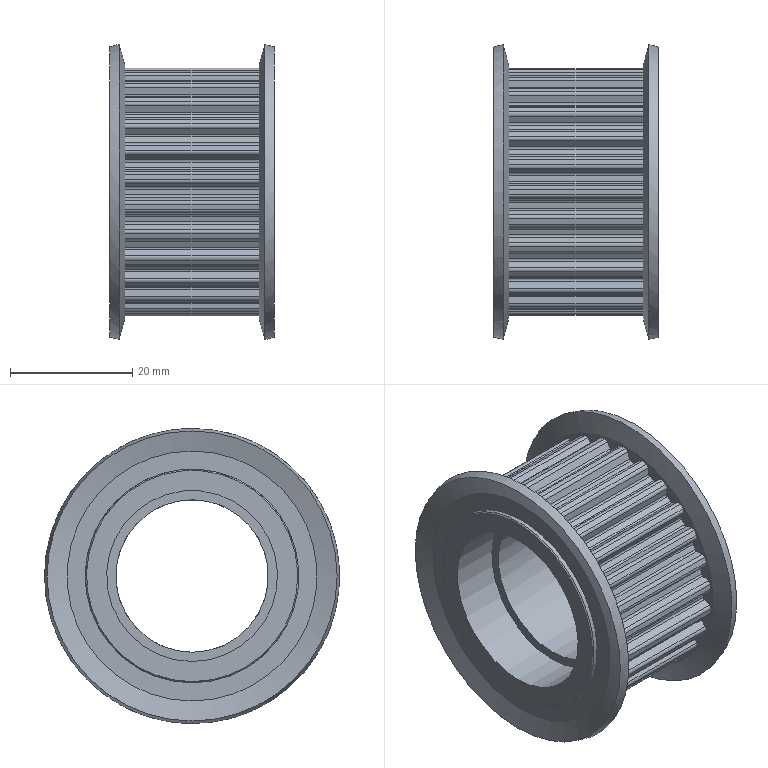Part | NX | 1 solid | 228 faces | box 27 x 48.354 x 48.354 mm | volume 18376 mm3 | cylinder 161 | plane 60 | cone 7 | commonest cylinder face diameters 0.8 x52 1.2 x52 37 x26 40.6 x26 28 x2 35 x2